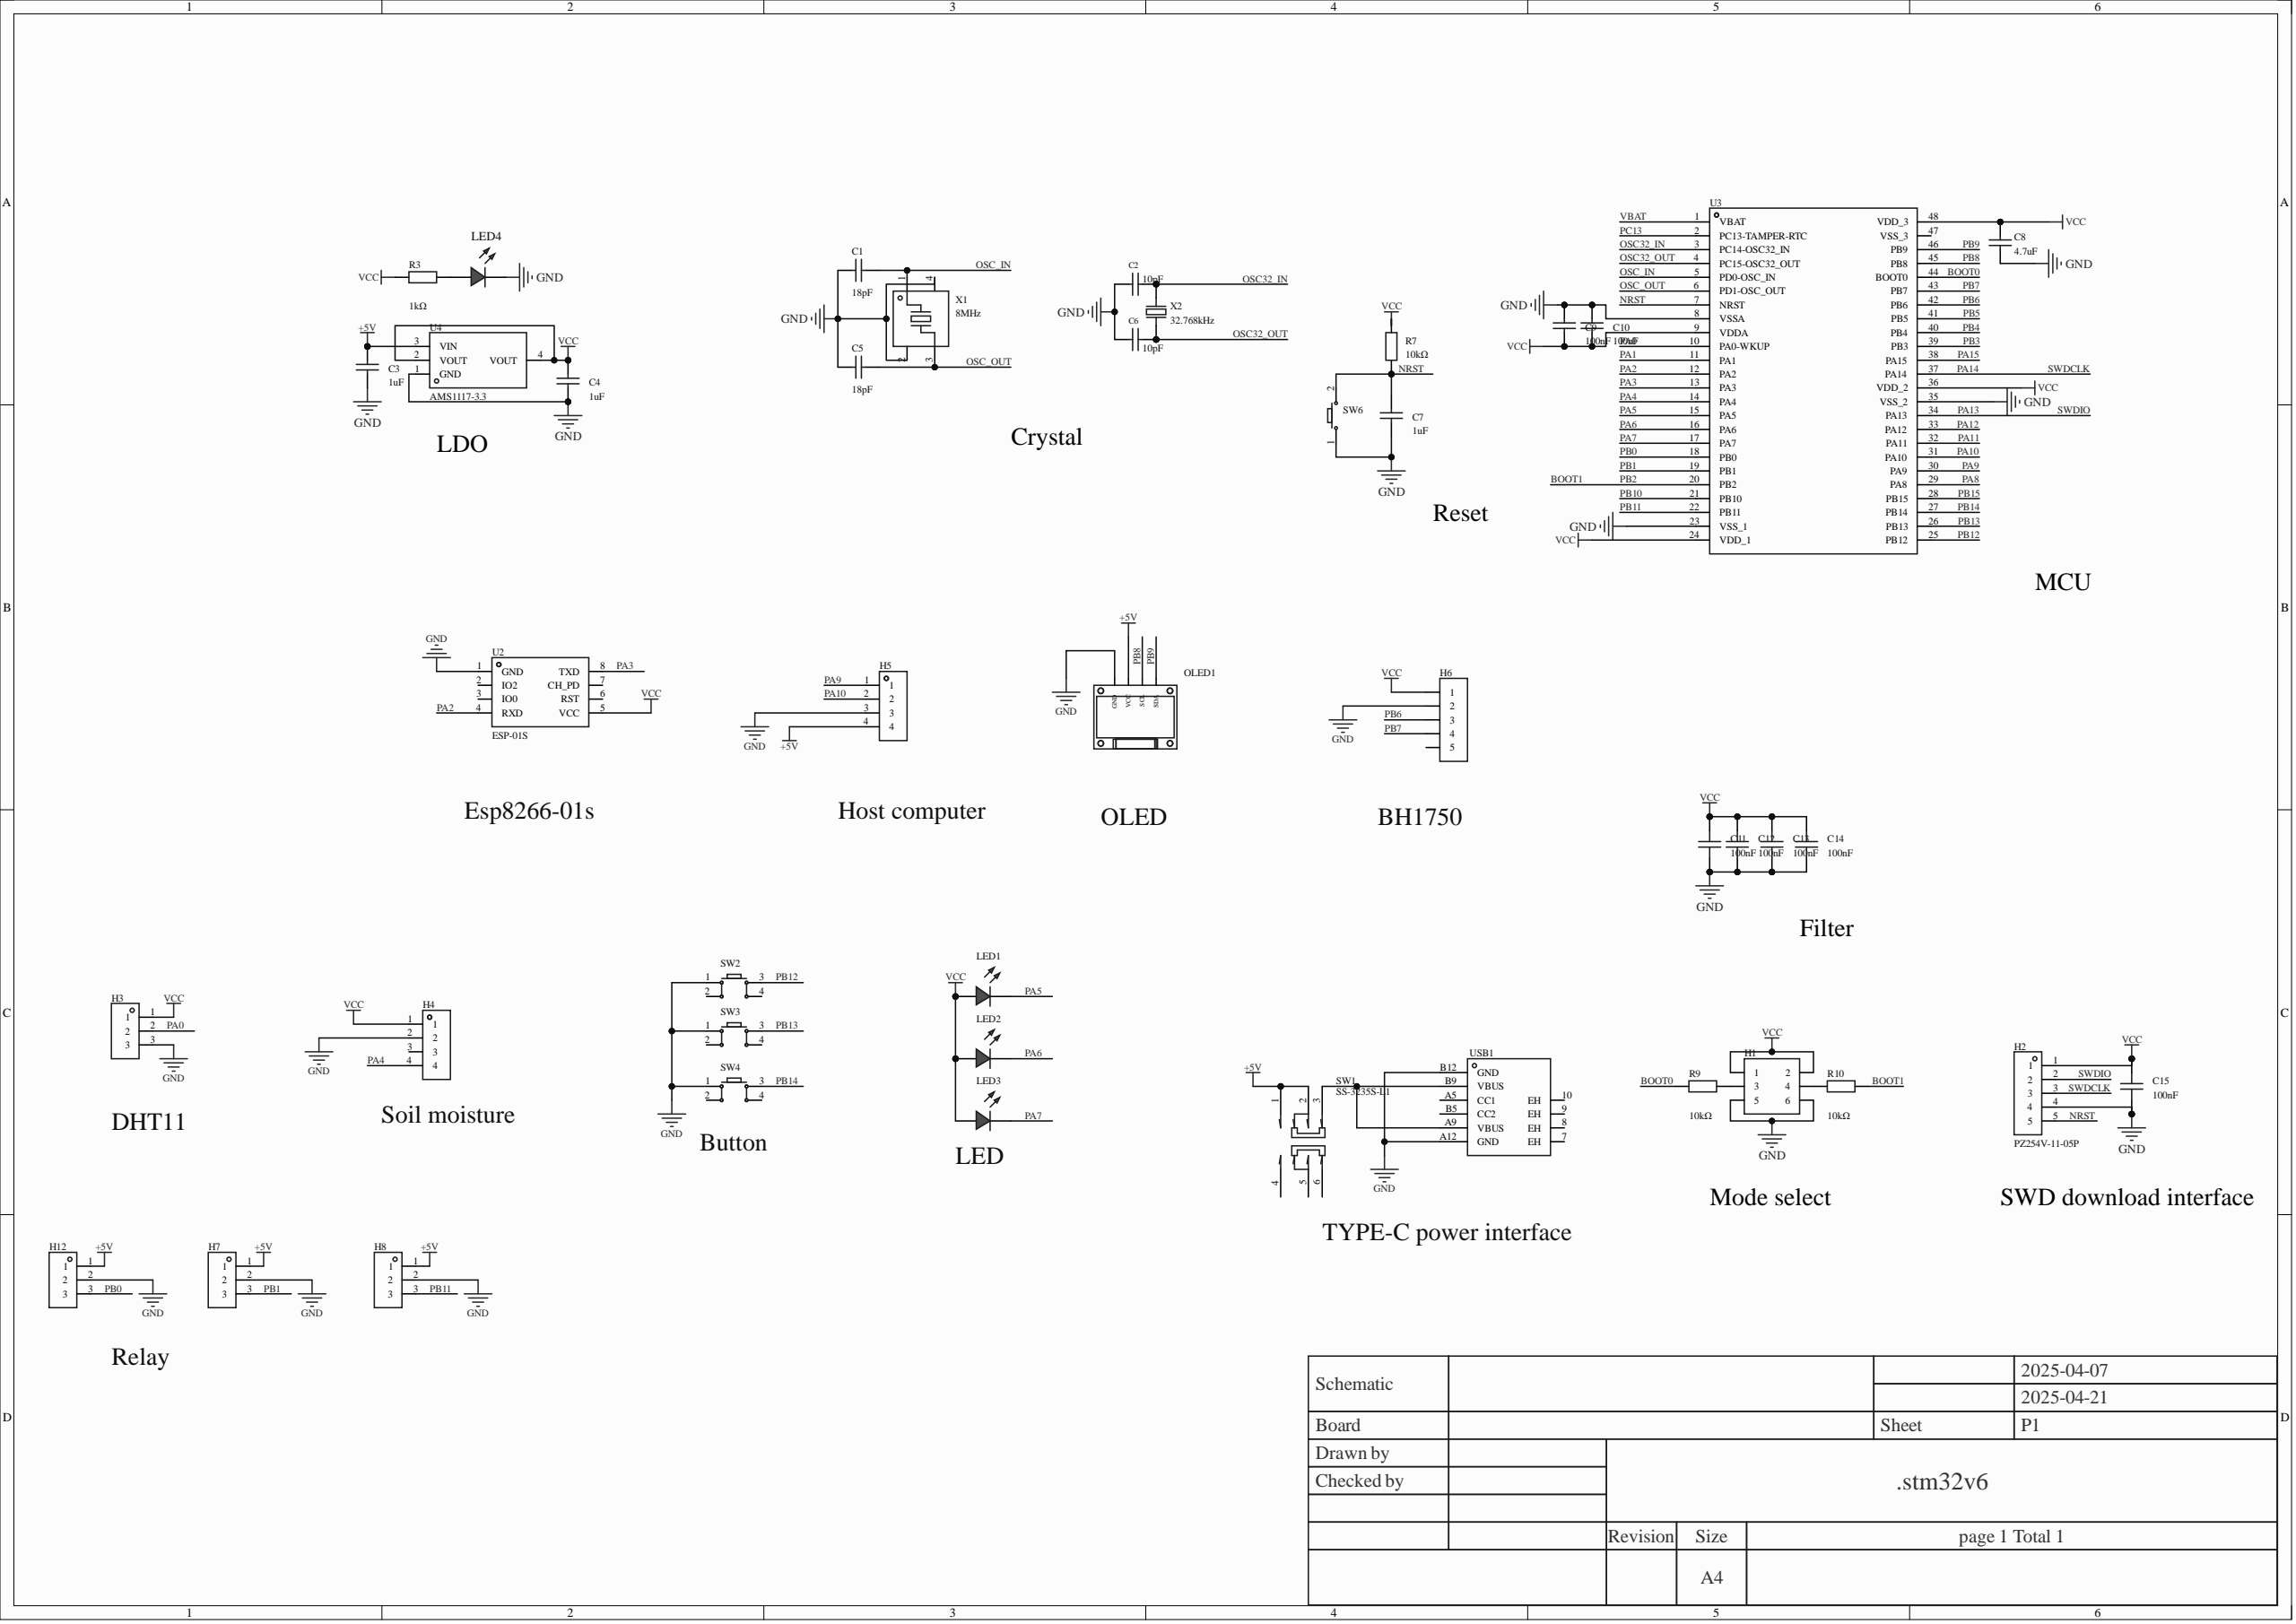Circuit board | Altium Designer | 44 parts | 35 nets
Bill of materials:
Comment,Description,Designator,Footprint,LibRef,Quantity
"18pF","Capacitance:18pF;Tolerance:±5%;Rated voltage:50V;Temperature coefficient:C0G;","C1, C5","C0805","FCC0603N180J500CT","2"
"10pF","Capacitance:10pF;Tolerance:±5%;Rated voltage:50V;Temperature coefficient:C0G;","C2, C6","C0805","CL10C100JB8NNNC","2"
"1uF","Capacitance:1uF;Tolerance:±10%;Rated voltage:10V;Dielectric (temperature coefficient):X5R;, Capacitance:1uF;Tolerance:±10%;Rated voltage:6.3V;Dielectric (temperature coefficient):X5R;, Capacitance:1uF;Tolerance:±10%;Rated voltage:50V;Temperature coefficient:X5R;","C3, C4, C7","C0805","CL05A105KP5NNNC, CL05A105KQ5NNNC, CGA0603X5R105K500JT","3"
"4.7uF","Capacitance:4.7uF;Tolerance:±10%;Rated voltage:16V;Temperature coefficient:X5R;","C8","C0805","CL10A475KO8NNNC","1"
"100nF","Capacitance:100nF;Tolerance:±10%;Rated voltage:50V;Temperature coefficient:X7R;","C9, C10, C11, C12, C13, C14, C15","C0805","CC0603KRX7R9BB104","7"
"","","H1","HDR-TH_6P-P2.54-V-R2-C3-S2.54_A2541WV-2X3P","HDR-M_2.54_2x3","1"
"PZ254V-11-05P","Pin structure:1x5P;Pitch:2.54mm;Row pitch:-;Round/square pin:Square pin;Mounting:Through-hole;Rows:Single row;Total pins:5P;Rated current:-;Rated voltage:-;Mating pin length:6mm;Insulator height:2.5mm;Tail length:3mm;Contact material:Brass;Contact plating:-;Operating temperature:-40℃~+105℃;Colour:Black;","H2","HDR-TH_5P-P2.54-V-M","PZ254V-11-05P","1"
"","","H3, H7, H8, H12","HDR-TH_3P-P2.54-V-F","HDR-F_2.54_1x3P","4"
"","","H4, H5","HDR-TH_4P-P2.54-V-F","HDR-F_2.54_1x4P","2"
"","","H6","HDR-TH_5P-P2.54-V-F","HDR-F_2.54_1x5P","1"
"","","LED1, LED2, LED3","LED_TH-3mm","LED_TH-R_3mm","3"
"","","LED4","LED_0402","LED_0402-R","1"
"","","OLED1","0.96OLED_4P","0.96OLED模块_4P","1"
"1kΩ","Resistor type:Thick film resistor;Resistance:1kΩ;Tolerance:±1%;Power:100mW;Max operating voltage:75V;Temperature coefficient:±100ppm/?;","R3","R0805","0603WAF1001T5E","1"
"10kΩ","Resistor type:Thick film resistor;Resistance:10kΩ;Tolerance:±1%;Power:100mW;Operating voltage:75V;Temperature coefficient:±100ppm/?;","R7, R9, R10","R0805","0603WAF1002T5E","3"
"SS-3235S-L1","Circuit structure:DPDT;Mounting:Horizontal SMD;Switch colour:Black;Rated current:50mA;Rated voltage:12V;Operating life:1 ten-thousand cycles;","SW1","SW-SMD_SS-3235S-LX","SS-3235S-L1","1"
"","","SW2, SW3, SW4","SW-TH_4P-L6.0-W6.0-P4.50-LS6.5","Key_TH_6x6x6","3"
"","","SW6","Key_SMD_3x4x2","Key_SMD_3x4x2","1"
"ESP-01S","","U2","WIFIM-TH_ESP-01S","ESP-01S_C111009","1"
"STM32F103C8T6","CPU core:CM3;Program memory capacity:64KB;Total RAM:20KB;GPIO count:37;Operating voltage range:2V~3.6V;Max CPU frequency:72MHz;Program memory type:FLASH;","U3","LQFP-48_L7.0-W7.0-P0.50-LS9.0-BL","STM32F103C8T6","1"
"AMS1117-3.3","Output type:Fixed;Operating voltage:-;Output voltage:3.3V;Output current:1A;Power supply rejection ratio (PSRR):72dB@(120Hz);Output polarity:Positive;","U4","SOT-223-3_L6.5-W3.4-P2.30-LS7.0-BR","AMS1117-3.3_C6186","1"
"","","USB1","USB_ TYPE-C-6P","USB_ Type-C-6P","1"
"8MHz","Crystal type:SMD crystal;Frequency:8MHz;Frequency tolerance (ambient):±10ppm;Load capacitance:12pF;Frequency stability (full temp.):±20ppm;","X1","OSC-SMD_4P-L3.2-W2.5-BL","X32258MOB4SI","1"
"32.768kHz","Crystal type:SMD crystal;Frequency:32.768kHz;Frequency tolerance (ambient):±20ppm;Load capacitance:6pF;","X2","CRYSTAL-SMD_L3.2-W1.5-1","Q13FC13500049","1"
Netlist (Protel format):
[
C1
C0805
18pF



]
[
C2
C0805
10pF



]
[
C3
C0805
1uF



]
[
C4
C0805
1uF



]
[
C5
C0805
18pF



]
[
C6
C0805
10pF



]
[
C7
C0805
1uF



]
[
C8
C0805
4.7uF



]
[
C9
C0805
100nF



]
[
C10
C0805
100nF



]
[
C11
C0805
100nF



]
[
C12
C0805
100nF



]
[
C13
C0805
100nF



]
[
C14
C0805
100nF



]
[
C15
C0805
100nF



]
[
H1
HDR-TH_6P-P2.54-V-R2-C3-S2.54_A2541WV-2X3P




]
[
H2
HDR-TH_5P-P2.54-V-M
PZ254V-11-05P



]
[
H3
HDR-TH_3P-P2.54-V-F




]
[
H4
HDR-TH_4P-P2.54-V-F




]
[
H5
HDR-TH_4P-P2.54-V-F




]
[
H6
HDR-TH_5P-P2.54-V-F




]
[
H7
HDR-TH_3P-P2.54-V-F




]
[
H8
HDR-TH_3P-P2.54-V-F




]
[
H12
HDR-TH_3P-P2.54-V-F




]
[
LED1
LED_TH-3mm




]
[
LED2
LED_TH-3mm




]
[
LED3
LED_TH-3mm




]
[
LED4
LED_0402




]
[
OLED1
0.96OLED_4P




]
[
R3
R0805
1kΩ



]
[
R7
R0805
10kΩ



]
[
R9
R0805
10kΩ



]
[
R10
R0805
10kΩ



]
[
SW1
SW-SMD_SS-3235S-LX
SS-3235S-L1



]
[
SW2
SW-TH_4P-L6.0-W6.0-P4.50-LS6.5




]
[
SW3
SW-TH_4P-L6.0-W6.0-P4.50-LS6.5




]
[
SW4
SW-TH_4P-L6.0-W6.0-P4.50-LS6.5




]
[
SW6
Key_SMD_3x4x2




]
[
U2
WIFIM-TH_ESP-01S
ESP-01S



]
[
U3
LQFP-48_L7.0-W7.0-P0.50-LS9.0-BL
STM32F103C8T6



]
[
U4
SOT-223-3_L6.5-W3.4-P2.30-LS7.0-BR
AMS1117-3.3



]
[
USB1
USB_ TYPE-C-6P




]
[
X1
OSC-SMD_4P-L3.2-W2.5-BL
8MHz



]
[
X2
CRYSTAL-SMD_L3.2-W1.5-1
32.768kHz



]
(
VCC
C4-2
C8-2
C9-1
C10-1
C11-2
C12-2
C13-2
C14-2
C15-2
H1-1
H1-2
H2-1
H3-1
H4-1
H6-1
LED1-1
LED2-1
LED3-1
R3-1
R7-2
U2-5
U3-9
U3-24
U3-36
U3-48
U4-2
U4-4
)
(
PB14
SW4-3
U3-27
)
(
PB13
SW3-3
U3-26
)
(
PB12
SW2-3
U3-25
)
(
PB11
H8-3
U3-22
)
(
PB9
OLED1-4
U3-46
)
(
PB8
OLED1-3
U3-45
)
(
PB7
H6-4
U3-43
)
(
PB6
H6-3
U3-42
)
(
PB1
H7-3
U3-19
)
(
PB0
H12-3
U3-18
)
(
PA14
H2-3
U3-37
)
(
PA13
H2-2
U3-34
)
(
PA10
H5-2
U3-31
)
(
PA9
H5-1
U3-30
)
(
PA7
LED3-2
U3-17
)
(
PA6
LED2-2
U3-16
)
(
PA5
LED1-2
U3-15
)
(
PA4
H4-4
U3-14
)
(
PA3
U2-8
U3-13
)
(
PA2
U2-4
U3-12
)
(
PA0
H3-2
U3-10
)
(
OSC_OUT
C5-1
U3-6
X1-3
)
(
OSC_IN
C1-1
U3-5
X1-1
)
(
OSC32_OUT
C6-2
U3-4
X2-1
)
(
OSC32_IN
C2-2
U3-3
X2-2
)
(
NRST
C7-1
H2-5
R7-1
SW6-2
U3-7
)
(
NetSW1_3
SW1-3
USB1-A9
USB1-B9
)
(
NetLED4_2
LED4-2
R3-2
)
(
NetH1_4
H1-4
R10-1
)
(
NetH1_3
H1-3
R9-2
)
(
GND
C1-2
C2-1
C3-1
C4-1
C5-2
C6-1
C7-2
C8-1
C9-2
C10-2
C11-1
C12-1
C13-1
C14-1
C15-1
H1-5
H1-6
H2-4
H3-3
H4-2
H5-3
H6-2
H7-2
H8-2
H12-2
LED4-1
OLED1-1
SW2-1
SW3-1
SW4-1
SW6-1
U2-1
U3-8
U3-23
U3-35
U4-1
USB1-A12
USB1-B12
X1-2
X1-4
)
(
BOOT1
R10-2
U3-20
)
(
BOOT0
R9-1
U3-44
)
(
+5V
C3-2
H5-4
H7-1
H8-1
H12-1
OLED1-2
SW1-1
SW1-2
U4-3
)